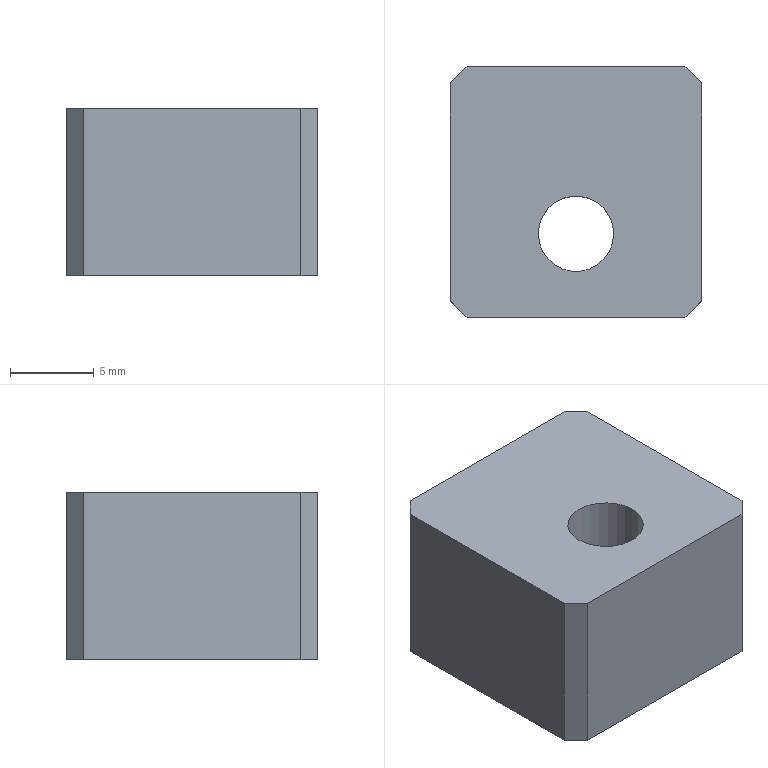Part | STEP file | 1_id1594_x_t | 1 solid | 13 faces | box 15 x 15 x 10 mm | volume 1899 mm3 | plane 11 | cylinder 2 | commonest cylinder face diameters 4.5 x1 8 x1
STEP:
#1=CARTESIAN_POINT('',(0.,0.,0.));
#2=DIRECTION('',(0.,0.,1.));
#3=DIRECTION('',(1.,0.,0.));
#4=AXIS2_PLACEMENT_3D('',#1,#2,#3);
#5=CARTESIAN_POINT('',(572.125,127.624,-49.278));
#6=VERTEX_POINT('',#5);
#7=CARTESIAN_POINT('',(572.125,127.624,-59.278));
#8=VERTEX_POINT('',#7);
#9=CARTESIAN_POINT('',(572.125,127.624,-49.278));
#10=DIRECTION('',(0.,0.,-1.));
#11=VECTOR('',#10,1.);
#12=LINE('',#9,#11);
#13=CARTESIAN_POINT('',(571.125,126.624,-49.278));
#14=DIRECTION('',(0.7071,-0.7071,0.));
#15=DIRECTION('',(0.,0.,1.));
#16=AXIS2_PLACEMENT_3D('',#13,#14,#15);
#17=PLANE('',#16);
#18=CARTESIAN_POINT('',(0.,-1.414));
#19=DIRECTION('',(-1.,0.));
#20=VECTOR('',#19,1.);
#21=LINE('',#18,#20);
#22=(GEOMETRIC_REPRESENTATION_CONTEXT(2)PARAMETRIC_REPRESENTATION_CONTEXT()REPRESENTATION_CONTEXT('',''));
#23=DEFINITIONAL_REPRESENTATION('',(#21),#22);
#24=PCURVE('',#17,#23);
#25=CARTESIAN_POINT('',(586.125,127.624,-49.278));
#26=DIRECTION('',(0.,-1.,0.));
#27=DIRECTION('',(-1.,0.,0.));
#28=AXIS2_PLACEMENT_3D('',#25,#26,#27);
#29=PLANE('',#28);
#30=CARTESIAN_POINT('',(14.,0.));
#31=DIRECTION('',(0.,1.));
#32=VECTOR('',#31,1.);
#33=LINE('',#30,#32);
#34=(GEOMETRIC_REPRESENTATION_CONTEXT(2)PARAMETRIC_REPRESENTATION_CONTEXT()REPRESENTATION_CONTEXT('',''));
#35=DEFINITIONAL_REPRESENTATION('',(#33),#34);
#36=PCURVE('',#29,#35);
#37=SURFACE_CURVE('',#12,(#24,#36),.PCURVE_S1.);
#38=EDGE_CURVE('',#6,#8,#37,.T.);
#39=ORIENTED_EDGE('',*,*,#38,.T.);
#40=CARTESIAN_POINT('',(571.125,126.624,-59.278));
#41=VERTEX_POINT('',#40);
#42=CARTESIAN_POINT('',(571.125,126.624,-59.278));
#43=DIRECTION('',(0.7071,0.7071,0.));
#44=VECTOR('',#43,1.);
#45=LINE('',#42,#44);
#46=CARTESIAN_POINT('',(-10.,0.));
#47=DIRECTION('',(0.,-1.));
#48=VECTOR('',#47,1.);
#49=LINE('',#46,#48);
#50=(GEOMETRIC_REPRESENTATION_CONTEXT(2)PARAMETRIC_REPRESENTATION_CONTEXT()REPRESENTATION_CONTEXT('',''));
#51=DEFINITIONAL_REPRESENTATION('',(#49),#50);
#52=PCURVE('',#17,#51);
#53=CARTESIAN_POINT('',(571.125,112.624,-59.278));
#54=DIRECTION('',(0.,0.,1.));
#55=DIRECTION('',(-1.,0.,0.));
#56=AXIS2_PLACEMENT_3D('',#53,#54,#55);
#57=PLANE('',#56);
#58=CARTESIAN_POINT('',(0.,-14.));
#59=DIRECTION('',(-0.7071,-0.7071));
#60=VECTOR('',#59,1.);
#61=LINE('',#58,#60);
#62=(GEOMETRIC_REPRESENTATION_CONTEXT(2)PARAMETRIC_REPRESENTATION_CONTEXT()REPRESENTATION_CONTEXT('',''));
#63=DEFINITIONAL_REPRESENTATION('',(#61),#62);
#64=PCURVE('',#57,#63);
#65=SURFACE_CURVE('',#45,(#52,#64),.PCURVE_S1.);
#66=EDGE_CURVE('',#41,#8,#65,.T.);
#67=ORIENTED_EDGE('',*,*,#66,.F.);
#68=CARTESIAN_POINT('',(571.125,126.624,-49.278));
#69=VERTEX_POINT('',#68);
#70=CARTESIAN_POINT('',(571.125,126.624,-59.278));
#71=DIRECTION('',(0.,0.,1.));
#72=VECTOR('',#71,1.);
#73=LINE('',#70,#72);
#74=CARTESIAN_POINT('',(-10.,0.));
#75=DIRECTION('',(1.,0.));
#76=VECTOR('',#75,1.);
#77=LINE('',#74,#76);
#78=(GEOMETRIC_REPRESENTATION_CONTEXT(2)PARAMETRIC_REPRESENTATION_CONTEXT()REPRESENTATION_CONTEXT('',''));
#79=DEFINITIONAL_REPRESENTATION('',(#77),#78);
#80=PCURVE('',#17,#79);
#81=CARTESIAN_POINT('',(571.125,127.624,-49.278));
#82=DIRECTION('',(1.,0.,0.));
#83=DIRECTION('',(0.,1.,0.));
#84=AXIS2_PLACEMENT_3D('',#81,#82,#83);
#85=PLANE('',#84);
#86=CARTESIAN_POINT('',(-1.,-10.));
#87=DIRECTION('',(0.,1.));
#88=VECTOR('',#87,1.);
#89=LINE('',#86,#88);
#90=(GEOMETRIC_REPRESENTATION_CONTEXT(2)PARAMETRIC_REPRESENTATION_CONTEXT()REPRESENTATION_CONTEXT('',''));
#91=DEFINITIONAL_REPRESENTATION('',(#89),#90);
#92=PCURVE('',#85,#91);
#93=SURFACE_CURVE('',#73,(#80,#92),.PCURVE_S1.);
#94=EDGE_CURVE('',#41,#69,#93,.T.);
#95=ORIENTED_EDGE('',*,*,#94,.T.);
#96=CARTESIAN_POINT('',(572.125,127.624,-49.278));
#97=DIRECTION('',(-0.7071,-0.7071,0.));
#98=VECTOR('',#97,1.);
#99=LINE('',#96,#98);
#100=CARTESIAN_POINT('',(0.,-1.414));
#101=DIRECTION('',(0.,1.));
#102=VECTOR('',#101,1.);
#103=LINE('',#100,#102);
#104=(GEOMETRIC_REPRESENTATION_CONTEXT(2)PARAMETRIC_REPRESENTATION_CONTEXT()REPRESENTATION_CONTEXT('',''));
#105=DEFINITIONAL_REPRESENTATION('',(#103),#104);
#106=PCURVE('',#17,#105);
#107=CARTESIAN_POINT('',(571.125,112.624,-49.278));
#108=DIRECTION('',(0.,0.,1.));
#109=DIRECTION('',(-1.,0.,0.));
#110=AXIS2_PLACEMENT_3D('',#107,#108,#109);
#111=PLANE('',#110);
#112=CARTESIAN_POINT('',(-1.,-15.));
#113=DIRECTION('',(0.7071,0.7071));
#114=VECTOR('',#113,1.);
#115=LINE('',#112,#114);
#116=(GEOMETRIC_REPRESENTATION_CONTEXT(2)PARAMETRIC_REPRESENTATION_CONTEXT()REPRESENTATION_CONTEXT('',''));
#117=DEFINITIONAL_REPRESENTATION('',(#115),#116);
#118=PCURVE('',#111,#117);
#119=SURFACE_CURVE('',#99,(#106,#118),.PCURVE_S1.);
#120=EDGE_CURVE('',#6,#69,#119,.T.);
#121=ORIENTED_EDGE('',*,*,#120,.F.);
#122=EDGE_LOOP('',(#39,#67,#95,#121));
#123=FACE_BOUND('',#122,.T.);
#124=ADVANCED_FACE('',(#123),#17,.F.);
#125=CARTESIAN_POINT('',(585.125,112.624,-49.278));
#126=VERTEX_POINT('',#125);
#127=CARTESIAN_POINT('',(586.125,113.624,-49.278));
#128=VERTEX_POINT('',#127);
#129=CARTESIAN_POINT('',(585.125,112.624,-49.278));
#130=DIRECTION('',(0.7071,0.7071,0.));
#131=VECTOR('',#130,1.);
#132=LINE('',#129,#131);
#133=CARTESIAN_POINT('',(-14.,0.));
#134=DIRECTION('',(-0.7071,-0.7071));
#135=VECTOR('',#134,1.);
#136=LINE('',#133,#135);
#137=(GEOMETRIC_REPRESENTATION_CONTEXT(2)PARAMETRIC_REPRESENTATION_CONTEXT()REPRESENTATION_CONTEXT('',''));
#138=DEFINITIONAL_REPRESENTATION('',(#136),#137);
#139=PCURVE('',#111,#138);
#140=CARTESIAN_POINT('',(586.125,113.624,-49.278));
#141=DIRECTION('',(-0.7071,0.7071,0.));
#142=DIRECTION('',(0.7071,0.7071,0.));
#143=AXIS2_PLACEMENT_3D('',#140,#141,#142);
#144=PLANE('',#143);
#145=CARTESIAN_POINT('',(-1.414,0.));
#146=DIRECTION('',(1.,0.));
#147=VECTOR('',#146,1.);
#148=LINE('',#145,#147);
#149=(GEOMETRIC_REPRESENTATION_CONTEXT(2)PARAMETRIC_REPRESENTATION_CONTEXT()REPRESENTATION_CONTEXT('',''));
#150=DEFINITIONAL_REPRESENTATION('',(#148),#149);
#151=PCURVE('',#144,#150);
#152=SURFACE_CURVE('',#132,(#139,#151),.PCURVE_S1.);
#153=EDGE_CURVE('',#126,#128,#152,.T.);
#154=ORIENTED_EDGE('',*,*,#153,.T.);
#155=CARTESIAN_POINT('',(586.125,126.624,-49.278));
#156=VERTEX_POINT('',#155);
#157=CARTESIAN_POINT('',(586.125,126.624,-49.278));
#158=DIRECTION('',(0.,-1.,0.));
#159=VECTOR('',#158,1.);
#160=LINE('',#157,#159);
#161=CARTESIAN_POINT('',(-15.,-14.));
#162=DIRECTION('',(0.,1.));
#163=VECTOR('',#162,1.);
#164=LINE('',#161,#163);
#165=(GEOMETRIC_REPRESENTATION_CONTEXT(2)PARAMETRIC_REPRESENTATION_CONTEXT()REPRESENTATION_CONTEXT('',''));
#166=DEFINITIONAL_REPRESENTATION('',(#164),#165);
#167=PCURVE('',#111,#166);
#168=CARTESIAN_POINT('',(586.125,112.624,-49.278));
#169=DIRECTION('',(-1.,0.,0.));
#170=DIRECTION('',(0.,0.,-1.));
#171=AXIS2_PLACEMENT_3D('',#168,#169,#170);
#172=PLANE('',#171);
#173=CARTESIAN_POINT('',(0.,-14.));
#174=DIRECTION('',(0.,1.));
#175=VECTOR('',#174,1.);
#176=LINE('',#173,#175);
#177=(GEOMETRIC_REPRESENTATION_CONTEXT(2)PARAMETRIC_REPRESENTATION_CONTEXT()REPRESENTATION_CONTEXT('',''));
#178=DEFINITIONAL_REPRESENTATION('',(#176),#177);
#179=PCURVE('',#172,#178);
#180=SURFACE_CURVE('',#160,(#167,#179),.PCURVE_S1.);
#181=EDGE_CURVE('',#156,#128,#180,.T.);
#182=ORIENTED_EDGE('',*,*,#181,.F.);
#183=CARTESIAN_POINT('',(585.125,127.624,-49.278));
#184=VERTEX_POINT('',#183);
#185=CARTESIAN_POINT('',(586.125,126.624,-49.278));
#186=DIRECTION('',(-0.7071,0.7071,0.));
#187=VECTOR('',#186,1.);
#188=LINE('',#185,#187);
#189=CARTESIAN_POINT('',(-15.,-14.));
#190=DIRECTION('',(0.7071,-0.7071));
#191=VECTOR('',#190,1.);
#192=LINE('',#189,#191);
#193=(GEOMETRIC_REPRESENTATION_CONTEXT(2)PARAMETRIC_REPRESENTATION_CONTEXT()REPRESENTATION_CONTEXT('',''));
#194=DEFINITIONAL_REPRESENTATION('',(#192),#193);
#195=PCURVE('',#111,#194);
#196=CARTESIAN_POINT('',(585.125,127.624,-49.278));
#197=DIRECTION('',(-0.7071,-0.7071,0.));
#198=DIRECTION('',(0.,0.,-1.));
#199=AXIS2_PLACEMENT_3D('',#196,#197,#198);
#200=PLANE('',#199);
#201=CARTESIAN_POINT('',(0.,1.414));
#202=DIRECTION('',(0.,-1.));
#203=VECTOR('',#202,1.);
#204=LINE('',#201,#203);
#205=(GEOMETRIC_REPRESENTATION_CONTEXT(2)PARAMETRIC_REPRESENTATION_CONTEXT()REPRESENTATION_CONTEXT('',''));
#206=DEFINITIONAL_REPRESENTATION('',(#204),#205);
#207=PCURVE('',#200,#206);
#208=SURFACE_CURVE('',#188,(#195,#207),.PCURVE_S1.);
#209=EDGE_CURVE('',#156,#184,#208,.T.);
#210=ORIENTED_EDGE('',*,*,#209,.T.);
#211=CARTESIAN_POINT('',(572.125,127.624,-49.278));
#212=DIRECTION('',(1.,0.,0.));
#213=VECTOR('',#212,1.);
#214=LINE('',#211,#213);
#215=CARTESIAN_POINT('',(-1.,-15.));
#216=DIRECTION('',(-1.,0.));
#217=VECTOR('',#216,1.);
#218=LINE('',#215,#217);
#219=(GEOMETRIC_REPRESENTATION_CONTEXT(2)PARAMETRIC_REPRESENTATION_CONTEXT()REPRESENTATION_CONTEXT('',''));
#220=DEFINITIONAL_REPRESENTATION('',(#218),#219);
#221=PCURVE('',#111,#220);
#222=CARTESIAN_POINT('',(14.,0.));
#223=DIRECTION('',(-1.,0.));
#224=VECTOR('',#223,1.);
#225=LINE('',#222,#224);
#226=(GEOMETRIC_REPRESENTATION_CONTEXT(2)PARAMETRIC_REPRESENTATION_CONTEXT()REPRESENTATION_CONTEXT('',''));
#227=DEFINITIONAL_REPRESENTATION('',(#225),#226);
#228=PCURVE('',#29,#227);
#229=SURFACE_CURVE('',#214,(#221,#228),.PCURVE_S1.);
#230=EDGE_CURVE('',#6,#184,#229,.T.);
#231=ORIENTED_EDGE('',*,*,#230,.F.);
#232=ORIENTED_EDGE('',*,*,#120,.T.);
#233=CARTESIAN_POINT('',(571.125,113.624,-49.278));
#234=VERTEX_POINT('',#233);
#235=CARTESIAN_POINT('',(571.125,113.624,-49.278));
#236=DIRECTION('',(0.,1.,0.));
#237=VECTOR('',#236,1.);
#238=LINE('',#235,#237);
#239=CARTESIAN_POINT('',(0.,-1.));
#240=DIRECTION('',(0.,-1.));
#241=VECTOR('',#240,1.);
#242=LINE('',#239,#241);
#243=(GEOMETRIC_REPRESENTATION_CONTEXT(2)PARAMETRIC_REPRESENTATION_CONTEXT()REPRESENTATION_CONTEXT('',''));
#244=DEFINITIONAL_REPRESENTATION('',(#242),#243);
#245=PCURVE('',#111,#244);
#246=CARTESIAN_POINT('',(-14.,0.));
#247=DIRECTION('',(1.,0.));
#248=VECTOR('',#247,1.);
#249=LINE('',#246,#248);
#250=(GEOMETRIC_REPRESENTATION_CONTEXT(2)PARAMETRIC_REPRESENTATION_CONTEXT()REPRESENTATION_CONTEXT('',''));
#251=DEFINITIONAL_REPRESENTATION('',(#249),#250);
#252=PCURVE('',#85,#251);
#253=SURFACE_CURVE('',#238,(#245,#252),.PCURVE_S1.);
#254=EDGE_CURVE('',#234,#69,#253,.T.);
#255=ORIENTED_EDGE('',*,*,#254,.F.);
#256=CARTESIAN_POINT('',(572.125,112.624,-49.278));
#257=VERTEX_POINT('',#256);
#258=CARTESIAN_POINT('',(571.125,113.624,-49.278));
#259=DIRECTION('',(0.7071,-0.7071,0.));
#260=VECTOR('',#259,1.);
#261=LINE('',#258,#260);
#262=CARTESIAN_POINT('',(0.,-1.));
#263=DIRECTION('',(-0.7071,0.7071));
#264=VECTOR('',#263,1.);
#265=LINE('',#262,#264);
#266=(GEOMETRIC_REPRESENTATION_CONTEXT(2)PARAMETRIC_REPRESENTATION_CONTEXT()REPRESENTATION_CONTEXT('',''));
#267=DEFINITIONAL_REPRESENTATION('',(#265),#266);
#268=PCURVE('',#111,#267);
#269=CARTESIAN_POINT('',(571.125,113.624,-49.278));
#270=DIRECTION('',(0.7071,0.7071,0.));
#271=DIRECTION('',(0.7071,-0.7071,0.));
#272=AXIS2_PLACEMENT_3D('',#269,#270,#271);
#273=PLANE('',#272);
#274=CARTESIAN_POINT('',(0.,0.));
#275=DIRECTION('',(1.,0.));
#276=VECTOR('',#275,1.);
#277=LINE('',#274,#276);
#278=(GEOMETRIC_REPRESENTATION_CONTEXT(2)PARAMETRIC_REPRESENTATION_CONTEXT()REPRESENTATION_CONTEXT('',''));
#279=DEFINITIONAL_REPRESENTATION('',(#277),#278);
#280=PCURVE('',#273,#279);
#281=SURFACE_CURVE('',#261,(#268,#280),.PCURVE_S1.);
#282=EDGE_CURVE('',#234,#257,#281,.T.);
#283=ORIENTED_EDGE('',*,*,#282,.T.);
#284=CARTESIAN_POINT('',(585.125,112.624,-49.278));
#285=DIRECTION('',(-1.,0.,0.));
#286=VECTOR('',#285,1.);
#287=LINE('',#284,#286);
#288=CARTESIAN_POINT('',(-14.,0.));
#289=DIRECTION('',(1.,0.));
#290=VECTOR('',#289,1.);
#291=LINE('',#288,#290);
#292=(GEOMETRIC_REPRESENTATION_CONTEXT(2)PARAMETRIC_REPRESENTATION_CONTEXT()REPRESENTATION_CONTEXT('',''));
#293=DEFINITIONAL_REPRESENTATION('',(#291),#292);
#294=PCURVE('',#111,#293);
#295=CARTESIAN_POINT('',(571.125,112.624,-49.278));
#296=DIRECTION('',(0.,1.,0.));
#297=DIRECTION('',(0.,0.,1.));
#298=AXIS2_PLACEMENT_3D('',#295,#296,#297);
#299=PLANE('',#298);
#300=CARTESIAN_POINT('',(0.,14.));
#301=DIRECTION('',(0.,-1.));
#302=VECTOR('',#301,1.);
#303=LINE('',#300,#302);
#304=(GEOMETRIC_REPRESENTATION_CONTEXT(2)PARAMETRIC_REPRESENTATION_CONTEXT()REPRESENTATION_CONTEXT('',''));
#305=DEFINITIONAL_REPRESENTATION('',(#303),#304);
#306=PCURVE('',#299,#305);
#307=SURFACE_CURVE('',#287,(#294,#306),.PCURVE_S1.);
#308=EDGE_CURVE('',#126,#257,#307,.T.);
#309=ORIENTED_EDGE('',*,*,#308,.F.);
#310=EDGE_LOOP('',(#154,#182,#210,#231,#232,#255,#283,#309));
#311=FACE_BOUND('',#310,.T.);
#312=CARTESIAN_POINT('',(580.875,117.624,-49.278));
#313=VERTEX_POINT('',#312);
#314=CARTESIAN_POINT('',(578.625,117.624,-49.278));
#315=DIRECTION('',(0.,0.,-1.));
#316=DIRECTION('',(1.,0.,0.));
#317=AXIS2_PLACEMENT_3D('',#314,#315,#316);
#318=CIRCLE('',#317,2.25);
#319=CARTESIAN_POINT('',(-9.75,-5.));
#320=CARTESIAN_POINT('',(-9.75,-1.103));
#321=CARTESIAN_POINT('',(-6.375,-3.051));
#322=CARTESIAN_POINT('',(-3.,-5.));
#323=CARTESIAN_POINT('',(-6.375,-6.949));
#324=CARTESIAN_POINT('',(-9.75,-8.897));
#325=CARTESIAN_POINT('',(-9.75,-5.));
#326=(BOUNDED_CURVE()B_SPLINE_CURVE(2,(#319,#320,#321,#322,#323,#324,#325),.UNSPECIFIED.,.T.,.F.)B_SPLINE_CURVE_WITH_KNOTS((1,2,2,2,2,1),(-2.094,0.,2.094,4.189,6.283,8.378),.UNSPECIFIED.)CURVE()GEOMETRIC_REPRESENTATION_ITEM()RATIONAL_B_SPLINE_CURVE((1.,0.5,1.,0.5,1.,0.5,1.))REPRESENTATION_ITEM(''));
#327=(GEOMETRIC_REPRESENTATION_CONTEXT(2)PARAMETRIC_REPRESENTATION_CONTEXT()REPRESENTATION_CONTEXT('',''));
#328=DEFINITIONAL_REPRESENTATION('',(#326),#327);
#329=PCURVE('',#111,#328);
#330=CARTESIAN_POINT('',(578.625,117.624,-47.028));
#331=DIRECTION('',(0.,0.,1.));
#332=DIRECTION('',(1.,0.,0.));
#333=AXIS2_PLACEMENT_3D('',#330,#331,#332);
#334=CYLINDRICAL_SURFACE('',#333,2.25);
#335=CARTESIAN_POINT('',(6.283,-2.25));
#336=DIRECTION('',(-1.,0.));
#337=VECTOR('',#336,1.);
#338=LINE('',#335,#337);
#339=(GEOMETRIC_REPRESENTATION_CONTEXT(2)PARAMETRIC_REPRESENTATION_CONTEXT()REPRESENTATION_CONTEXT('',''));
#340=DEFINITIONAL_REPRESENTATION('',(#338),#339);
#341=PCURVE('',#334,#340);
#342=SURFACE_CURVE('',#318,(#329,#341),.PCURVE_S1.);
#343=EDGE_CURVE('',#313,#313,#342,.T.);
#344=ORIENTED_EDGE('',*,*,#343,.T.);
#345=EDGE_LOOP('',(#344));
#346=FACE_BOUND('',#345,.T.);
#347=ADVANCED_FACE('',(#311,#346),#111,.T.);
#348=CARTESIAN_POINT('',(585.125,112.624,-59.278));
#349=VERTEX_POINT('',#348);
#350=CARTESIAN_POINT('',(585.125,112.624,-59.278));
#351=DIRECTION('',(0.,0.,1.));
#352=VECTOR('',#351,1.);
#353=LINE('',#350,#352);
#354=CARTESIAN_POINT('',(-10.,14.));
#355=DIRECTION('',(1.,0.));
#356=VECTOR('',#355,1.);
#357=LINE('',#354,#356);
#358=(GEOMETRIC_REPRESENTATION_CONTEXT(2)PARAMETRIC_REPRESENTATION_CONTEXT()REPRESENTATION_CONTEXT('',''));
#359=DEFINITIONAL_REPRESENTATION('',(#357),#358);
#360=PCURVE('',#299,#359);
#361=CARTESIAN_POINT('',(-1.414,10.));
#362=DIRECTION('',(0.,-1.));
#363=VECTOR('',#362,1.);
#364=LINE('',#361,#363);
#365=(GEOMETRIC_REPRESENTATION_CONTEXT(2)PARAMETRIC_REPRESENTATION_CONTEXT()REPRESENTATION_CONTEXT('',''));
#366=DEFINITIONAL_REPRESENTATION('',(#364),#365);
#367=PCURVE('',#144,#366);
#368=SURFACE_CURVE('',#353,(#360,#367),.PCURVE_S1.);
#369=EDGE_CURVE('',#349,#126,#368,.T.);
#370=ORIENTED_EDGE('',*,*,#369,.T.);
#371=ORIENTED_EDGE('',*,*,#308,.T.);
#372=CARTESIAN_POINT('',(572.125,112.624,-59.278));
#373=VERTEX_POINT('',#372);
#374=CARTESIAN_POINT('',(572.125,112.624,-49.278));
#375=DIRECTION('',(0.,0.,-1.));
#376=VECTOR('',#375,1.);
#377=LINE('',#374,#376);
#378=CARTESIAN_POINT('',(0.,1.));
#379=DIRECTION('',(-1.,0.));
#380=VECTOR('',#379,1.);
#381=LINE('',#378,#380);
#382=(GEOMETRIC_REPRESENTATION_CONTEXT(2)PARAMETRIC_REPRESENTATION_CONTEXT()REPRESENTATION_CONTEXT('',''));
#383=DEFINITIONAL_REPRESENTATION('',(#381),#382);
#384=PCURVE('',#299,#383);
#385=CARTESIAN_POINT('',(1.414,0.));
#386=DIRECTION('',(0.,1.));
#387=VECTOR('',#386,1.);
#388=LINE('',#385,#387);
#389=(GEOMETRIC_REPRESENTATION_CONTEXT(2)PARAMETRIC_REPRESENTATION_CONTEXT()REPRESENTATION_CONTEXT('',''));
#390=DEFINITIONAL_REPRESENTATION('',(#388),#389);
#391=PCURVE('',#273,#390);
#392=SURFACE_CURVE('',#377,(#384,#391),.PCURVE_S1.);
#393=EDGE_CURVE('',#257,#373,#392,.T.);
#394=ORIENTED_EDGE('',*,*,#393,.T.);
#395=CARTESIAN_POINT('',(585.125,112.624,-59.278));
#396=DIRECTION('',(-1.,0.,0.));
#397=VECTOR('',#396,1.);
#398=LINE('',#395,#397);
#399=CARTESIAN_POINT('',(-10.,14.));
#400=DIRECTION('',(0.,-1.));
#401=VECTOR('',#400,1.);
#402=LINE('',#399,#401);
#403=(GEOMETRIC_REPRESENTATION_CONTEXT(2)PARAMETRIC_REPRESENTATION_CONTEXT()REPRESENTATION_CONTEXT('',''));
#404=DEFINITIONAL_REPRESENTATION('',(#402),#403);
#405=PCURVE('',#299,#404);
#406=CARTESIAN_POINT('',(-14.,0.));
#407=DIRECTION('',(1.,0.));
#408=VECTOR('',#407,1.);
#409=LINE('',#406,#408);
#410=(GEOMETRIC_REPRESENTATION_CONTEXT(2)PARAMETRIC_REPRESENTATION_CONTEXT()REPRESENTATION_CONTEXT('',''));
#411=DEFINITIONAL_REPRESENTATION('',(#409),#410);
#412=PCURVE('',#57,#411);
#413=SURFACE_CURVE('',#398,(#405,#412),.PCURVE_S1.);
#414=EDGE_CURVE('',#349,#373,#413,.T.);
#415=ORIENTED_EDGE('',*,*,#414,.F.);
#416=EDGE_LOOP('',(#370,#371,#394,#415));
#417=FACE_BOUND('',#416,.T.);
#418=ADVANCED_FACE('',(#417),#299,.F.);
#419=ORIENTED_EDGE('',*,*,#66,.T.);
#420=CARTESIAN_POINT('',(585.125,127.624,-59.278));
#421=VERTEX_POINT('',#420);
#422=CARTESIAN_POINT('',(572.125,127.624,-59.278));
#423=DIRECTION('',(1.,0.,0.));
#424=VECTOR('',#423,1.);
#425=LINE('',#422,#424);
#426=CARTESIAN_POINT('',(-1.,-15.));
#427=DIRECTION('',(-1.,0.));
#428=VECTOR('',#427,1.);
#429=LINE('',#426,#428);
#430=(GEOMETRIC_REPRESENTATION_CONTEXT(2)PARAMETRIC_REPRESENTATION_CONTEXT()REPRESENTATION_CONTEXT('',''));
#431=DEFINITIONAL_REPRESENTATION('',(#429),#430);
#432=PCURVE('',#57,#431);
#433=CARTESIAN_POINT('',(14.,10.));
#434=DIRECTION('',(-1.,0.));
#435=VECTOR('',#434,1.);
#436=LINE('',#433,#435);
#437=(GEOMETRIC_REPRESENTATION_CONTEXT(2)PARAMETRIC_REPRESENTATION_CONTEXT()REPRESENTATION_CONTEXT('',''));
#438=DEFINITIONAL_REPRESENTATION('',(#436),#437);
#439=PCURVE('',#29,#438);
#440=SURFACE_CURVE('',#425,(#432,#439),.PCURVE_S1.);
#441=EDGE_CURVE('',#8,#421,#440,.T.);
#442=ORIENTED_EDGE('',*,*,#441,.T.);
#443=CARTESIAN_POINT('',(586.125,126.624,-59.278));
#444=VERTEX_POINT('',#443);
#445=CARTESIAN_POINT('',(585.125,127.624,-59.278));
#446=DIRECTION('',(0.7071,-0.7071,0.));
#447=VECTOR('',#446,1.);
#448=LINE('',#445,#447);
#449=CARTESIAN_POINT('',(-14.,-15.));
#450=DIRECTION('',(-0.7071,0.7071));
#451=VECTOR('',#450,1.);
#452=LINE('',#449,#451);
#453=(GEOMETRIC_REPRESENTATION_CONTEXT(2)PARAMETRIC_REPRESENTATION_CONTEXT()REPRESENTATION_CONTEXT('',''));
#454=DEFINITIONAL_REPRESENTATION('',(#452),#453);
#455=PCURVE('',#57,#454);
#456=CARTESIAN_POINT('',(10.,0.));
#457=DIRECTION('',(0.,1.));
#458=VECTOR('',#457,1.);
#459=LINE('',#456,#458);
#460=(GEOMETRIC_REPRESENTATION_CONTEXT(2)PARAMETRIC_REPRESENTATION_CONTEXT()REPRESENTATION_CONTEXT('',''));
#461=DEFINITIONAL_REPRESENTATION('',(#459),#460);
#462=PCURVE('',#200,#461);
#463=SURFACE_CURVE('',#448,(#455,#462),.PCURVE_S1.);
#464=EDGE_CURVE('',#421,#444,#463,.T.);
#465=ORIENTED_EDGE('',*,*,#464,.T.);
#466=CARTESIAN_POINT('',(586.125,113.624,-59.278));
#467=VERTEX_POINT('',#466);
#468=CARTESIAN_POINT('',(586.125,126.624,-59.278));
#469=DIRECTION('',(0.,-1.,0.));
#470=VECTOR('',#469,1.);
#471=LINE('',#468,#470);
#472=CARTESIAN_POINT('',(-15.,-14.));
#473=DIRECTION('',(0.,1.));
#474=VECTOR('',#473,1.);
#475=LINE('',#472,#474);
#476=(GEOMETRIC_REPRESENTATION_CONTEXT(2)PARAMETRIC_REPRESENTATION_CONTEXT()REPRESENTATION_CONTEXT('',''));
#477=DEFINITIONAL_REPRESENTATION('',(#475),#476);
#478=PCURVE('',#57,#477);
#479=CARTESIAN_POINT('',(10.,-14.));
#480=DIRECTION('',(0.,1.));
#481=VECTOR('',#480,1.);
#482=LINE('',#479,#481);
#483=(GEOMETRIC_REPRESENTATION_CONTEXT(2)PARAMETRIC_REPRESENTATION_CONTEXT()REPRESENTATION_CONTEXT('',''));
#484=DEFINITIONAL_REPRESENTATION('',(#482),#483);
#485=PCURVE('',#172,#484);
#486=SURFACE_CURVE('',#471,(#478,#485),.PCURVE_S1.);
#487=EDGE_CURVE('',#444,#467,#486,.T.);
#488=ORIENTED_EDGE('',*,*,#487,.T.);
#489=CARTESIAN_POINT('',(586.125,113.624,-59.278));
#490=DIRECTION('',(-0.7071,-0.7071,0.));
#491=VECTOR('',#490,1.);
#492=LINE('',#489,#491);
#493=CARTESIAN_POINT('',(-15.,-1.));
#494=DIRECTION('',(0.7071,0.7071));
#495=VECTOR('',#494,1.);
#496=LINE('',#493,#495);
#497=(GEOMETRIC_REPRESENTATION_CONTEXT(2)PARAMETRIC_REPRESENTATION_CONTEXT()REPRESENTATION_CONTEXT('',''));
#498=DEFINITIONAL_REPRESENTATION('',(#496),#497);
#499=PCURVE('',#57,#498);
#500=CARTESIAN_POINT('',(0.,10.));
#501=DIRECTION('',(-1.,0.));
#502=VECTOR('',#501,1.);
#503=LINE('',#500,#502);
#504=(GEOMETRIC_REPRESENTATION_CONTEXT(2)PARAMETRIC_REPRESENTATION_CONTEXT()REPRESENTATION_CONTEXT('',''));
#505=DEFINITIONAL_REPRESENTATION('',(#503),#504);
#506=PCURVE('',#144,#505);
#507=SURFACE_CURVE('',#492,(#499,#506),.PCURVE_S1.);
#508=EDGE_CURVE('',#467,#349,#507,.T.);
#509=ORIENTED_EDGE('',*,*,#508,.T.);
#510=ORIENTED_EDGE('',*,*,#414,.T.);
#511=CARTESIAN_POINT('',(571.125,113.624,-59.278));
#512=VERTEX_POINT('',#511);
#513=CARTESIAN_POINT('',(572.125,112.624,-59.278));
#514=DIRECTION('',(-0.7071,0.7071,0.));
#515=VECTOR('',#514,1.);
#516=LINE('',#513,#515);
#517=CARTESIAN_POINT('',(-1.,0.));
#518=DIRECTION('',(0.7071,-0.7071));
#519=VECTOR('',#518,1.);
#520=LINE('',#517,#519);
#521=(GEOMETRIC_REPRESENTATION_CONTEXT(2)PARAMETRIC_REPRESENTATION_CONTEXT()REPRESENTATION_CONTEXT('',''));
#522=DEFINITIONAL_REPRESENTATION('',(#520),#521);
#523=PCURVE('',#57,#522);
#524=CARTESIAN_POINT('',(1.414,10.));
#525=DIRECTION('',(-1.,0.));
#526=VECTOR('',#525,1.);
#527=LINE('',#524,#526);
#528=(GEOMETRIC_REPRESENTATION_CONTEXT(2)PARAMETRIC_REPRESENTATION_CONTEXT()REPRESENTATION_CONTEXT('',''));
#529=DEFINITIONAL_REPRESENTATION('',(#527),#528);
#530=PCURVE('',#273,#529);
#531=SURFACE_CURVE('',#516,(#523,#530),.PCURVE_S1.);
#532=EDGE_CURVE('',#373,#512,#531,.T.);
#533=ORIENTED_EDGE('',*,*,#532,.T.);
#534=CARTESIAN_POINT('',(571.125,113.624,-59.278));
#535=DIRECTION('',(0.,1.,0.));
#536=VECTOR('',#535,1.);
#537=LINE('',#534,#536);
#538=CARTESIAN_POINT('',(0.,-1.));
#539=DIRECTION('',(0.,-1.));
#540=VECTOR('',#539,1.);
#541=LINE('',#538,#540);
#542=(GEOMETRIC_REPRESENTATION_CONTEXT(2)PARAMETRIC_REPRESENTATION_CONTEXT()REPRESENTATION_CONTEXT('',''));
#543=DEFINITIONAL_REPRESENTATION('',(#541),#542);
#544=PCURVE('',#57,#543);
#545=CARTESIAN_POINT('',(-14.,-10.));
#546=DIRECTION('',(1.,0.));
#547=VECTOR('',#546,1.);
#548=LINE('',#545,#547);
#549=(GEOMETRIC_REPRESENTATION_CONTEXT(2)PARAMETRIC_REPRESENTATION_CONTEXT()REPRESENTATION_CONTEXT('',''));
#550=DEFINITIONAL_REPRESENTATION('',(#548),#549);
#551=PCURVE('',#85,#550);
#552=SURFACE_CURVE('',#537,(#544,#551),.PCURVE_S1.);
#553=EDGE_CURVE('',#512,#41,#552,.T.);
#554=ORIENTED_EDGE('',*,*,#553,.T.);
#555=EDGE_LOOP('',(#419,#442,#465,#488,#509,#510,#533,#554));
#556=FACE_BOUND('',#555,.T.);
#557=CARTESIAN_POINT('',(574.625,117.624,-59.278));
#558=VERTEX_POINT('',#557);
#559=CARTESIAN_POINT('',(582.625,117.624,-59.278));
#560=VERTEX_POINT('',#559);
#561=CARTESIAN_POINT('',(578.625,117.624,-59.278));
#562=DIRECTION('',(0.,0.,1.));
#563=DIRECTION('',(-1.,0.,0.));
#564=AXIS2_PLACEMENT_3D('',#561,#562,#563);
#565=CIRCLE('',#564,4.);
#566=CARTESIAN_POINT('',(-7.5,-5.));
#567=DIRECTION('',(1.,0.));
#568=AXIS2_PLACEMENT_2D('',#566,#567);
#569=CIRCLE('',#568,4.);
#570=(GEOMETRIC_REPRESENTATION_CONTEXT(2)PARAMETRIC_REPRESENTATION_CONTEXT()REPRESENTATION_CONTEXT('',''));
#571=DEFINITIONAL_REPRESENTATION('',(#569),#570);
#572=PCURVE('',#57,#571);
#573=CARTESIAN_POINT('',(578.625,117.624,-54.278));
#574=DIRECTION('',(0.,0.,1.));
#575=DIRECTION('',(1.,0.,0.));
#576=AXIS2_PLACEMENT_3D('',#573,#574,#575);
#577=CYLINDRICAL_SURFACE('',#576,4.);
#578=CARTESIAN_POINT('',(3.142,-5.));
#579=DIRECTION('',(1.,0.));
#580=VECTOR('',#579,1.);
#581=LINE('',#578,#580);
#582=(GEOMETRIC_REPRESENTATION_CONTEXT(2)PARAMETRIC_REPRESENTATION_CONTEXT()REPRESENTATION_CONTEXT('',''));
#583=DEFINITIONAL_REPRESENTATION('',(#581),#582);
#584=PCURVE('',#577,#583);
#585=SURFACE_CURVE('',#565,(#572,#584),.PCURVE_S1.);
#586=EDGE_CURVE('',#558,#560,#585,.T.);
#587=ORIENTED_EDGE('',*,*,#586,.T.);
#588=CARTESIAN_POINT('',(578.625,117.624,-59.278));
#589=DIRECTION('',(0.,0.,1.));
#590=DIRECTION('',(-1.,0.,0.));
#591=AXIS2_PLACEMENT_3D('',#588,#589,#590);
#592=CIRCLE('',#591,4.);
#593=CARTESIAN_POINT('',(-7.5,-5.));
#594=DIRECTION('',(1.,0.));
#595=AXIS2_PLACEMENT_2D('',#593,#594);
#596=CIRCLE('',#595,4.);
#597=(GEOMETRIC_REPRESENTATION_CONTEXT(2)PARAMETRIC_REPRESENTATION_CONTEXT()REPRESENTATION_CONTEXT('',''));
#598=DEFINITIONAL_REPRESENTATION('',(#596),#597);
#599=PCURVE('',#57,#598);
#600=CARTESIAN_POINT('',(-3.142,-5.));
#601=DIRECTION('',(1.,0.));
#602=VECTOR('',#601,1.);
#603=LINE('',#600,#602);
#604=(GEOMETRIC_REPRESENTATION_CONTEXT(2)PARAMETRIC_REPRESENTATION_CONTEXT()REPRESENTATION_CONTEXT('',''));
#605=DEFINITIONAL_REPRESENTATION('',(#603),#604);
#606=PCURVE('',#577,#605);
#607=SURFACE_CURVE('',#592,(#599,#606),.PCURVE_S1.);
#608=EDGE_CURVE('',#560,#558,#607,.T.);
#609=ORIENTED_EDGE('',*,*,#608,.T.);
#610=EDGE_LOOP('',(#587,#609));
#611=FACE_BOUND('',#610,.T.);
#612=ADVANCED_FACE('',(#556,#611),#57,.F.);
#613=ORIENTED_EDGE('',*,*,#94,.F.);
#614=ORIENTED_EDGE('',*,*,#553,.F.);
#615=CARTESIAN_POINT('',(571.125,113.624,-59.278));
#616=DIRECTION('',(0.,0.,1.));
#617=VECTOR('',#616,1.);
#618=LINE('',#615,#617);
#619=CARTESIAN_POINT('',(-14.,-10.));
#620=DIRECTION('',(0.,1.));
#621=VECTOR('',#620,1.);
#622=LINE('',#619,#621);
#623=(GEOMETRIC_REPRESENTATION_CONTEXT(2)PARAMETRIC_REPRESENTATION_CONTEXT()REPRESENTATION_CONTEXT('',''));
#624=DEFINITIONAL_REPRESENTATION('',(#622),#623);
#625=PCURVE('',#85,#624);
#626=CARTESIAN_POINT('',(0.,10.));
#627=DIRECTION('',(0.,-1.));
#628=VECTOR('',#627,1.);
#629=LINE('',#626,#628);
#630=(GEOMETRIC_REPRESENTATION_CONTEXT(2)PARAMETRIC_REPRESENTATION_CONTEXT()REPRESENTATION_CONTEXT('',''));
#631=DEFINITIONAL_REPRESENTATION('',(#629),#630);
#632=PCURVE('',#273,#631);
#633=SURFACE_CURVE('',#618,(#625,#632),.PCURVE_S1.);
#634=EDGE_CURVE('',#512,#234,#633,.T.);
#635=ORIENTED_EDGE('',*,*,#634,.T.);
#636=ORIENTED_EDGE('',*,*,#254,.T.);
#637=EDGE_LOOP('',(#613,#614,#635,#636));
#638=FACE_BOUND('',#637,.T.);
#639=ADVANCED_FACE('',(#638),#85,.F.);
#640=ORIENTED_EDGE('',*,*,#634,.F.);
#641=ORIENTED_EDGE('',*,*,#532,.F.);
#642=ORIENTED_EDGE('',*,*,#393,.F.);
#643=ORIENTED_EDGE('',*,*,#282,.F.);
#644=EDGE_LOOP('',(#640,#641,#642,#643));
#645=FACE_BOUND('',#644,.T.);
#646=ADVANCED_FACE('',(#645),#273,.F.);
#647=CARTESIAN_POINT('',(586.125,113.624,-49.278));
#648=DIRECTION('',(0.,0.,-1.));
#649=VECTOR('',#648,1.);
#650=LINE('',#647,#649);
#651=CARTESIAN_POINT('',(0.,0.));
#652=DIRECTION('',(0.,1.));
#653=VECTOR('',#652,1.);
#654=LINE('',#651,#653);
#655=(GEOMETRIC_REPRESENTATION_CONTEXT(2)PARAMETRIC_REPRESENTATION_CONTEXT()REPRESENTATION_CONTEXT('',''));
#656=DEFINITIONAL_REPRESENTATION('',(#654),#655);
#657=PCURVE('',#144,#656);
#658=CARTESIAN_POINT('',(0.,-1.));
#659=DIRECTION('',(1.,0.));
#660=VECTOR('',#659,1.);
#661=LINE('',#658,#660);
#662=(GEOMETRIC_REPRESENTATION_CONTEXT(2)PARAMETRIC_REPRESENTATION_CONTEXT()REPRESENTATION_CONTEXT('',''));
#663=DEFINITIONAL_REPRESENTATION('',(#661),#662);
#664=PCURVE('',#172,#663);
#665=SURFACE_CURVE('',#650,(#657,#664),.PCURVE_S1.);
#666=EDGE_CURVE('',#128,#467,#665,.T.);
#667=ORIENTED_EDGE('',*,*,#666,.F.);
#668=ORIENTED_EDGE('',*,*,#153,.F.);
#669=ORIENTED_EDGE('',*,*,#369,.F.);
#670=ORIENTED_EDGE('',*,*,#508,.F.);
#671=EDGE_LOOP('',(#667,#668,#669,#670));
#672=FACE_BOUND('',#671,.T.);
#673=ADVANCED_FACE('',(#672),#144,.F.);
#674=CARTESIAN_POINT('',(586.125,126.624,-49.278));
#675=DIRECTION('',(0.,0.,-1.));
#676=VECTOR('',#675,1.);
#677=LINE('',#674,#676);
#678=CARTESIAN_POINT('',(0.,-14.));
#679=DIRECTION('',(1.,0.));
#680=VECTOR('',#679,1.);
#681=LINE('',#678,#680);
#682=(GEOMETRIC_REPRESENTATION_CONTEXT(2)PARAMETRIC_REPRESENTATION_CONTEXT()REPRESENTATION_CONTEXT('',''));
#683=DEFINITIONAL_REPRESENTATION('',(#681),#682);
#684=PCURVE('',#172,#683);
#685=CARTESIAN_POINT('',(0.,1.414));
#686=DIRECTION('',(1.,0.));
#687=VECTOR('',#686,1.);
#688=LINE('',#685,#687);
#689=(GEOMETRIC_REPRESENTATION_CONTEXT(2)PARAMETRIC_REPRESENTATION_CONTEXT()REPRESENTATION_CONTEXT('',''));
#690=DEFINITIONAL_REPRESENTATION('',(#688),#689);
#691=PCURVE('',#200,#690);
#692=SURFACE_CURVE('',#677,(#684,#691),.PCURVE_S1.);
#693=EDGE_CURVE('',#156,#444,#692,.T.);
#694=ORIENTED_EDGE('',*,*,#693,.F.);
#695=ORIENTED_EDGE('',*,*,#181,.T.);
#696=ORIENTED_EDGE('',*,*,#666,.T.);
#697=ORIENTED_EDGE('',*,*,#487,.F.);
#698=EDGE_LOOP('',(#694,#695,#696,#697));
#699=FACE_BOUND('',#698,.T.);
#700=ADVANCED_FACE('',(#699),#172,.F.);
#701=ORIENTED_EDGE('',*,*,#693,.T.);
#702=ORIENTED_EDGE('',*,*,#464,.F.);
#703=CARTESIAN_POINT('',(585.125,127.624,-59.278));
#704=DIRECTION('',(0.,0.,1.));
#705=VECTOR('',#704,1.);
#706=LINE('',#703,#705);
#707=CARTESIAN_POINT('',(10.,0.));
#708=DIRECTION('',(-1.,0.));
#709=VECTOR('',#708,1.);
#710=LINE('',#707,#709);
#711=(GEOMETRIC_REPRESENTATION_CONTEXT(2)PARAMETRIC_REPRESENTATION_CONTEXT()REPRESENTATION_CONTEXT('',''));
#712=DEFINITIONAL_REPRESENTATION('',(#710),#711);
#713=PCURVE('',#200,#712);
#714=CARTESIAN_POINT('',(1.,10.));
#715=DIRECTION('',(0.,-1.));
#716=VECTOR('',#715,1.);
#717=LINE('',#714,#716);
#718=(GEOMETRIC_REPRESENTATION_CONTEXT(2)PARAMETRIC_REPRESENTATION_CONTEXT()REPRESENTATION_CONTEXT('',''));
#719=DEFINITIONAL_REPRESENTATION('',(#717),#718);
#720=PCURVE('',#29,#719);
#721=SURFACE_CURVE('',#706,(#713,#720),.PCURVE_S1.);
#722=EDGE_CURVE('',#421,#184,#721,.T.);
#723=ORIENTED_EDGE('',*,*,#722,.T.);
#724=ORIENTED_EDGE('',*,*,#209,.F.);
#725=EDGE_LOOP('',(#701,#702,#723,#724));
#726=FACE_BOUND('',#725,.T.);
#727=ADVANCED_FACE('',(#726),#200,.F.);
#728=ORIENTED_EDGE('',*,*,#38,.F.);
#729=ORIENTED_EDGE('',*,*,#230,.T.);
#730=ORIENTED_EDGE('',*,*,#722,.F.);
#731=ORIENTED_EDGE('',*,*,#441,.F.);
#732=EDGE_LOOP('',(#728,#729,#730,#731));
#733=FACE_BOUND('',#732,.T.);
#734=ADVANCED_FACE('',(#733),#29,.F.);
#735=CARTESIAN_POINT('',(582.625,117.624,-54.278));
#736=VERTEX_POINT('',#735);
#737=CARTESIAN_POINT('',(578.625,117.624,-54.278));
#738=DIRECTION('',(0.,0.,-1.));
#739=DIRECTION('',(1.,0.,0.));
#740=AXIS2_PLACEMENT_3D('',#737,#738,#739);
#741=CIRCLE('',#740,4.);
#742=CARTESIAN_POINT('',(6.283,0.));
#743=DIRECTION('',(-1.,0.));
#744=VECTOR('',#743,1.);
#745=LINE('',#742,#744);
#746=(GEOMETRIC_REPRESENTATION_CONTEXT(2)PARAMETRIC_REPRESENTATION_CONTEXT()REPRESENTATION_CONTEXT('',''));
#747=DEFINITIONAL_REPRESENTATION('',(#745),#746);
#748=PCURVE('',#577,#747);
#749=CARTESIAN_POINT('',(578.625,117.624,-54.278));
#750=DIRECTION('',(0.,0.,1.));
#751=DIRECTION('',(-1.,0.,0.));
#752=AXIS2_PLACEMENT_3D('',#749,#750,#751);
#753=PLANE('',#752);
#754=CARTESIAN_POINT('',(-4.,0.));
#755=CARTESIAN_POINT('',(-4.,6.928));
#756=CARTESIAN_POINT('',(2.,3.464));
#757=CARTESIAN_POINT('',(8.,0.));
#758=CARTESIAN_POINT('',(2.,-3.464));
#759=CARTESIAN_POINT('',(-4.,-6.928));
#760=CARTESIAN_POINT('',(-4.,0.));
#761=(BOUNDED_CURVE()B_SPLINE_CURVE(2,(#754,#755,#756,#757,#758,#759,#760),.UNSPECIFIED.,.T.,.F.)B_SPLINE_CURVE_WITH_KNOTS((1,2,2,2,2,1),(-2.094,0.,2.094,4.189,6.283,8.378),.UNSPECIFIED.)CURVE()GEOMETRIC_REPRESENTATION_ITEM()RATIONAL_B_SPLINE_CURVE((1.,0.5,1.,0.5,1.,0.5,1.))REPRESENTATION_ITEM(''));
#762=(GEOMETRIC_REPRESENTATION_CONTEXT(2)PARAMETRIC_REPRESENTATION_CONTEXT()REPRESENTATION_CONTEXT('',''));
#763=DEFINITIONAL_REPRESENTATION('',(#761),#762);
#764=PCURVE('',#753,#763);
#765=SURFACE_CURVE('',#741,(#748,#764),.PCURVE_S1.);
#766=EDGE_CURVE('',#736,#736,#765,.T.);
#767=ORIENTED_EDGE('',*,*,#766,.T.);
#768=CARTESIAN_POINT('',(582.625,117.624,-59.278));
#769=CARTESIAN_POINT('',(582.625,117.624,-54.278));
#770=B_SPLINE_CURVE_WITH_KNOTS('',1,(#768,#769),.UNSPECIFIED.,.F.,.F.,(2,2),(-5.,0.),.PIECEWISE_BEZIER_KNOTS.);
#771=CARTESIAN_POINT('',(0.,0.));
#772=DIRECTION('',(0.,1.));
#773=VECTOR('',#772,1.);
#774=LINE('',#771,#773);
#775=(GEOMETRIC_REPRESENTATION_CONTEXT(2)PARAMETRIC_REPRESENTATION_CONTEXT()REPRESENTATION_CONTEXT('',''));
#776=DEFINITIONAL_REPRESENTATION('',(#774),#775);
#777=PCURVE('',#577,#776);
#778=CARTESIAN_POINT('',(6.283,0.));
#779=DIRECTION('',(0.,1.));
#780=VECTOR('',#779,1.);
#781=LINE('',#778,#780);
#782=(GEOMETRIC_REPRESENTATION_CONTEXT(2)PARAMETRIC_REPRESENTATION_CONTEXT()REPRESENTATION_CONTEXT('',''));
#783=DEFINITIONAL_REPRESENTATION('',(#781),#782);
#784=PCURVE('',#577,#783);
#785=SEAM_CURVE('',#770,(#777,#784),.PCURVE_S1.);
#786=EDGE_CURVE('',#560,#736,#785,.T.);
#787=ORIENTED_EDGE('',*,*,#786,.F.);
#788=ORIENTED_EDGE('',*,*,#608,.T.);
#789=ORIENTED_EDGE('',*,*,#586,.T.);
#790=ORIENTED_EDGE('',*,*,#786,.T.);
#791=EDGE_LOOP('',(#767,#787,#788,#789,#790));
#792=FACE_BOUND('',#791,.F.);
#793=ADVANCED_FACE('',(#792),#577,.F.);
#794=ORIENTED_EDGE('',*,*,#766,.T.);
#795=EDGE_LOOP('',(#794));
#796=FACE_BOUND('',#795,.T.);
#797=CARTESIAN_POINT('',(580.875,117.624,-54.278));
#798=VERTEX_POINT('',#797);
#799=CARTESIAN_POINT('',(578.625,117.624,-54.278));
#800=DIRECTION('',(0.,0.,1.));
#801=DIRECTION('',(1.,0.,0.));
#802=AXIS2_PLACEMENT_3D('',#799,#800,#801);
#803=CIRCLE('',#802,2.25);
#804=CARTESIAN_POINT('',(0.,0.));
#805=DIRECTION('',(-1.,0.));
#806=AXIS2_PLACEMENT_2D('',#804,#805);
#807=CIRCLE('',#806,2.25);
#808=(GEOMETRIC_REPRESENTATION_CONTEXT(2)PARAMETRIC_REPRESENTATION_CONTEXT()REPRESENTATION_CONTEXT('',''));
#809=DEFINITIONAL_REPRESENTATION('',(#807),#808);
#810=PCURVE('',#753,#809);
#811=CARTESIAN_POINT('',(0.,-7.25));
#812=DIRECTION('',(1.,0.));
#813=VECTOR('',#812,1.);
#814=LINE('',#811,#813);
#815=(GEOMETRIC_REPRESENTATION_CONTEXT(2)PARAMETRIC_REPRESENTATION_CONTEXT()REPRESENTATION_CONTEXT('',''));
#816=DEFINITIONAL_REPRESENTATION('',(#814),#815);
#817=PCURVE('',#334,#816);
#818=SURFACE_CURVE('',#803,(#810,#817),.PCURVE_S1.);
#819=EDGE_CURVE('',#798,#798,#818,.T.);
#820=ORIENTED_EDGE('',*,*,#819,.T.);
#821=EDGE_LOOP('',(#820));
#822=FACE_BOUND('',#821,.T.);
#823=ADVANCED_FACE('',(#796,#822),#753,.F.);
#824=ORIENTED_EDGE('',*,*,#343,.T.);
#825=CARTESIAN_POINT('',(580.875,117.624,-54.278));
#826=CARTESIAN_POINT('',(580.875,117.624,-49.278));
#827=B_SPLINE_CURVE_WITH_KNOTS('',1,(#825,#826),.UNSPECIFIED.,.F.,.F.,(2,2),(-7.25,-2.25),.PIECEWISE_BEZIER_KNOTS.);
#828=CARTESIAN_POINT('',(0.,0.));
#829=DIRECTION('',(0.,1.));
#830=VECTOR('',#829,1.);
#831=LINE('',#828,#830);
#832=(GEOMETRIC_REPRESENTATION_CONTEXT(2)PARAMETRIC_REPRESENTATION_CONTEXT()REPRESENTATION_CONTEXT('',''));
#833=DEFINITIONAL_REPRESENTATION('',(#831),#832);
#834=PCURVE('',#334,#833);
#835=CARTESIAN_POINT('',(6.283,0.));
#836=DIRECTION('',(0.,1.));
#837=VECTOR('',#836,1.);
#838=LINE('',#835,#837);
#839=(GEOMETRIC_REPRESENTATION_CONTEXT(2)PARAMETRIC_REPRESENTATION_CONTEXT()REPRESENTATION_CONTEXT('',''));
#840=DEFINITIONAL_REPRESENTATION('',(#838),#839);
#841=PCURVE('',#334,#840);
#842=SEAM_CURVE('',#827,(#834,#841),.PCURVE_S1.);
#843=EDGE_CURVE('',#798,#313,#842,.T.);
#844=ORIENTED_EDGE('',*,*,#843,.F.);
#845=ORIENTED_EDGE('',*,*,#819,.T.);
#846=ORIENTED_EDGE('',*,*,#843,.T.);
#847=EDGE_LOOP('',(#824,#844,#845,#846));
#848=FACE_BOUND('',#847,.F.);
#849=ADVANCED_FACE('',(#848),#334,.F.);
#850=CLOSED_SHELL('',(#124,#347,#418,#612,#639,#646,#673,#700,#727,#734,#793,#823,#849));
#851=MANIFOLD_SOLID_BREP('',#850);
#852=(LENGTH_UNIT()NAMED_UNIT(*)SI_UNIT(.MILLI.,.METRE.));
#853=UNCERTAINTY_MEASURE_WITH_UNIT(LENGTH_MEASURE(0.000002),#852,'','');
#854=(NAMED_UNIT(*)PLANE_ANGLE_UNIT()SI_UNIT($,.RADIAN.));
#855=(NAMED_UNIT(*)SI_UNIT($,.STERADIAN.)SOLID_ANGLE_UNIT());
#856=(GEOMETRIC_REPRESENTATION_CONTEXT(3)GLOBAL_UNCERTAINTY_ASSIGNED_CONTEXT((#853))GLOBAL_UNIT_ASSIGNED_CONTEXT((#852,#854,#855))REPRESENTATION_CONTEXT('',''));
#857=ADVANCED_BREP_SHAPE_REPRESENTATION('',(#4,#851),#856);